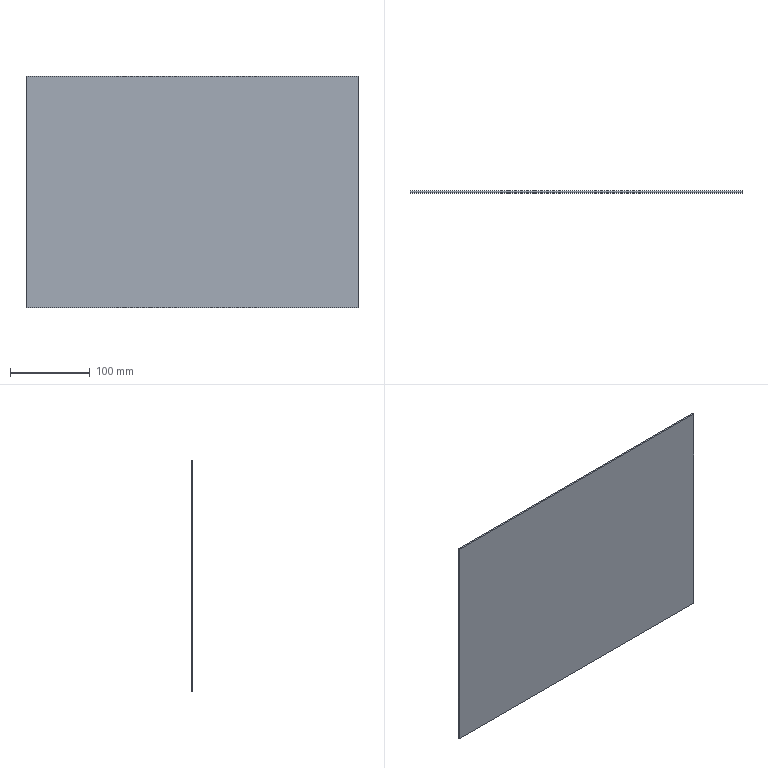Part | SolidWorks | features Extrusion 1 | 1 solid | 6 faces | box 415.5 x 2 x 290 mm | volume 240990 mm3 | plane 6
STEP:
#1=CARTESIAN_POINT('',(207.75,0.,145.));
#2=VERTEX_POINT('',#1);
#3=CARTESIAN_POINT('',(207.75,0.,-145.));
#4=VERTEX_POINT('',#3);
#5=CARTESIAN_POINT('',(207.75,0.,145.));
#6=DIRECTION('',(0.,0.,-1.));
#7=VECTOR('',#6,1000.);
#8=LINE('',#5,#7);
#9=EDGE_CURVE('',#2,#4,#8,.T.);
#10=ORIENTED_EDGE('',*,*,#9,.T.);
#11=CARTESIAN_POINT('',(207.75,2.,-145.));
#12=VERTEX_POINT('',#11);
#13=CARTESIAN_POINT('',(207.75,2.,-145.));
#14=DIRECTION('',(0.,-1.,0.));
#15=VECTOR('',#14,1000.);
#16=LINE('',#13,#15);
#17=EDGE_CURVE('',#12,#4,#16,.T.);
#18=ORIENTED_EDGE('',*,*,#17,.F.);
#19=CARTESIAN_POINT('',(207.75,2.,145.));
#20=VERTEX_POINT('',#19);
#21=CARTESIAN_POINT('',(207.75,2.,145.));
#22=DIRECTION('',(0.,0.,-1.));
#23=VECTOR('',#22,1000.);
#24=LINE('',#21,#23);
#25=EDGE_CURVE('',#20,#12,#24,.T.);
#26=ORIENTED_EDGE('',*,*,#25,.F.);
#27=CARTESIAN_POINT('',(207.75,2.,145.));
#28=DIRECTION('',(0.,-1.,0.));
#29=VECTOR('',#28,1000.);
#30=LINE('',#27,#29);
#31=EDGE_CURVE('',#20,#2,#30,.T.);
#32=ORIENTED_EDGE('',*,*,#31,.T.);
#33=EDGE_LOOP('',(#10,#18,#26,#32));
#34=FACE_OUTER_BOUND('',#33,.T.);
#35=CARTESIAN_POINT('',(207.75,2.,145.));
#36=DIRECTION('',(-1.,0.,0.));
#37=DIRECTION('',(0.,0.,1.));
#38=AXIS2_PLACEMENT_3D('',#35,#36,#37);
#39=PLANE('',#38);
#40=ADVANCED_FACE('',(#34),#39,.F.);
#41=CARTESIAN_POINT('',(-207.75,0.,-145.));
#42=VERTEX_POINT('',#41);
#43=CARTESIAN_POINT('',(-207.75,0.,-145.));
#44=DIRECTION('',(-1.,0.,0.));
#45=VECTOR('',#44,1000.);
#46=LINE('',#43,#45);
#47=EDGE_CURVE('',#4,#42,#46,.T.);
#48=ORIENTED_EDGE('',*,*,#47,.T.);
#49=CARTESIAN_POINT('',(-207.75,2.,-145.));
#50=VERTEX_POINT('',#49);
#51=CARTESIAN_POINT('',(-207.75,2.,-145.));
#52=DIRECTION('',(0.,-1.,0.));
#53=VECTOR('',#52,1000.);
#54=LINE('',#51,#53);
#55=EDGE_CURVE('',#50,#42,#54,.T.);
#56=ORIENTED_EDGE('',*,*,#55,.F.);
#57=CARTESIAN_POINT('',(-207.75,2.,-145.));
#58=DIRECTION('',(-1.,0.,0.));
#59=VECTOR('',#58,1000.);
#60=LINE('',#57,#59);
#61=EDGE_CURVE('',#12,#50,#60,.T.);
#62=ORIENTED_EDGE('',*,*,#61,.F.);
#63=ORIENTED_EDGE('',*,*,#17,.T.);
#64=EDGE_LOOP('',(#48,#56,#62,#63));
#65=FACE_OUTER_BOUND('',#64,.T.);
#66=CARTESIAN_POINT('',(-207.75,2.,-145.));
#67=DIRECTION('',(0.,0.,1.));
#68=DIRECTION('',(1.,0.,0.));
#69=AXIS2_PLACEMENT_3D('',#66,#67,#68);
#70=PLANE('',#69);
#71=ADVANCED_FACE('',(#65),#70,.F.);
#72=CARTESIAN_POINT('',(-207.75,0.,145.));
#73=VERTEX_POINT('',#72);
#74=CARTESIAN_POINT('',(-207.75,0.,145.));
#75=DIRECTION('',(0.,0.,1.));
#76=VECTOR('',#75,1000.);
#77=LINE('',#74,#76);
#78=EDGE_CURVE('',#42,#73,#77,.T.);
#79=ORIENTED_EDGE('',*,*,#78,.T.);
#80=CARTESIAN_POINT('',(-207.75,2.,145.));
#81=VERTEX_POINT('',#80);
#82=CARTESIAN_POINT('',(-207.75,2.,145.));
#83=DIRECTION('',(0.,-1.,0.));
#84=VECTOR('',#83,1000.);
#85=LINE('',#82,#84);
#86=EDGE_CURVE('',#81,#73,#85,.T.);
#87=ORIENTED_EDGE('',*,*,#86,.F.);
#88=CARTESIAN_POINT('',(-207.75,2.,145.));
#89=DIRECTION('',(0.,0.,1.));
#90=VECTOR('',#89,1000.);
#91=LINE('',#88,#90);
#92=EDGE_CURVE('',#50,#81,#91,.T.);
#93=ORIENTED_EDGE('',*,*,#92,.F.);
#94=ORIENTED_EDGE('',*,*,#55,.T.);
#95=EDGE_LOOP('',(#79,#87,#93,#94));
#96=FACE_OUTER_BOUND('',#95,.T.);
#97=CARTESIAN_POINT('',(-207.75,2.,145.));
#98=DIRECTION('',(1.,0.,0.));
#99=DIRECTION('',(0.,0.,-1.));
#100=AXIS2_PLACEMENT_3D('',#97,#98,#99);
#101=PLANE('',#100);
#102=ADVANCED_FACE('',(#96),#101,.F.);
#103=CARTESIAN_POINT('',(-207.75,0.,145.));
#104=DIRECTION('',(1.,0.,0.));
#105=VECTOR('',#104,1000.);
#106=LINE('',#103,#105);
#107=EDGE_CURVE('',#73,#2,#106,.T.);
#108=ORIENTED_EDGE('',*,*,#107,.T.);
#109=ORIENTED_EDGE('',*,*,#31,.F.);
#110=CARTESIAN_POINT('',(-207.75,2.,145.));
#111=DIRECTION('',(1.,0.,0.));
#112=VECTOR('',#111,1000.);
#113=LINE('',#110,#112);
#114=EDGE_CURVE('',#81,#20,#113,.T.);
#115=ORIENTED_EDGE('',*,*,#114,.F.);
#116=ORIENTED_EDGE('',*,*,#86,.T.);
#117=EDGE_LOOP('',(#108,#109,#115,#116));
#118=FACE_OUTER_BOUND('',#117,.T.);
#119=CARTESIAN_POINT('',(-207.75,2.,145.));
#120=DIRECTION('',(0.,0.,-1.));
#121=DIRECTION('',(-1.,0.,0.));
#122=AXIS2_PLACEMENT_3D('',#119,#120,#121);
#123=PLANE('',#122);
#124=ADVANCED_FACE('',(#118),#123,.F.);
#125=ORIENTED_EDGE('',*,*,#25,.T.);
#126=ORIENTED_EDGE('',*,*,#61,.T.);
#127=ORIENTED_EDGE('',*,*,#92,.T.);
#128=ORIENTED_EDGE('',*,*,#114,.T.);
#129=EDGE_LOOP('',(#125,#126,#127,#128));
#130=FACE_OUTER_BOUND('',#129,.T.);
#131=CARTESIAN_POINT('',(0.,2.,0.));
#132=DIRECTION('',(0.,-1.,0.));
#133=DIRECTION('',(0.,0.,-1.));
#134=AXIS2_PLACEMENT_3D('',#131,#132,#133);
#135=PLANE('',#134);
#136=ADVANCED_FACE('',(#130),#135,.F.);
#137=ORIENTED_EDGE('',*,*,#9,.F.);
#138=ORIENTED_EDGE('',*,*,#107,.F.);
#139=ORIENTED_EDGE('',*,*,#78,.F.);
#140=ORIENTED_EDGE('',*,*,#47,.F.);
#141=EDGE_LOOP('',(#137,#138,#139,#140));
#142=FACE_OUTER_BOUND('',#141,.T.);
#143=CARTESIAN_POINT('',(0.,0.,0.));
#144=DIRECTION('',(0.,-1.,0.));
#145=DIRECTION('',(0.,0.,-1.));
#146=AXIS2_PLACEMENT_3D('',#143,#144,#145);
#147=PLANE('',#146);
#148=ADVANCED_FACE('',(#142),#147,.T.);
#149=CLOSED_SHELL('',(#40,#71,#102,#124,#136,#148));
#150=MANIFOLD_SOLID_BREP('',#149);
#151=CARTESIAN_POINT('',(0.,0.,0.));
#152=DIRECTION('',(0.,0.,1.));
#153=DIRECTION('',(1.,0.,0.));
#154=AXIS2_PLACEMENT_3D('',#151,#152,#153);
#155=(LENGTH_UNIT()NAMED_UNIT(*)SI_UNIT(.MILLI.,.METRE.));
#156=UNCERTAINTY_MEASURE_WITH_UNIT(LENGTH_MEASURE(0.00001),#155,'','');
#157=(NAMED_UNIT(*)PLANE_ANGLE_UNIT()SI_UNIT($,.RADIAN.));
#158=(NAMED_UNIT(*)SI_UNIT($,.STERADIAN.)SOLID_ANGLE_UNIT());
#159=(GEOMETRIC_REPRESENTATION_CONTEXT(3)GLOBAL_UNCERTAINTY_ASSIGNED_CONTEXT((#156))GLOBAL_UNIT_ASSIGNED_CONTEXT((#155,#157,#158))REPRESENTATION_CONTEXT('',''));
#160=ADVANCED_BREP_SHAPE_REPRESENTATION('',(#150,#154),#159);